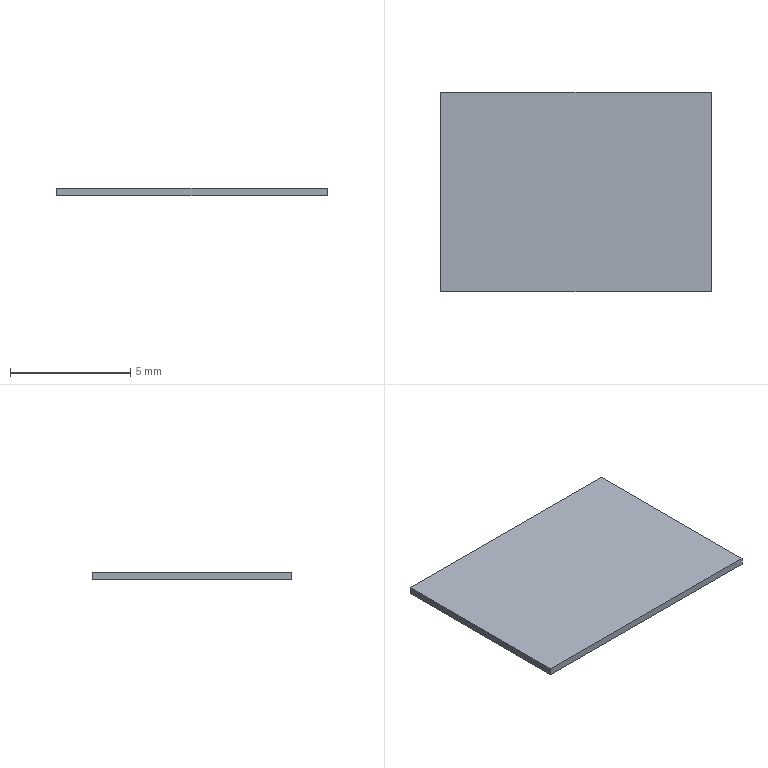Part | SolidWorks | features Extrusion 1 | 1 solid | 6 faces | box 11.25 x 8.29 x 0.3 mm | volume 27.979 mm3 | plane 6
STEP:
#1=CARTESIAN_POINT('',(5.625,-4.145,-0.15));
#2=VERTEX_POINT('',#1);
#3=CARTESIAN_POINT('',(5.625,4.145,-0.15));
#4=VERTEX_POINT('',#3);
#5=CARTESIAN_POINT('',(5.625,-4.145,-0.15));
#6=DIRECTION('',(0.,1.,0.));
#7=VECTOR('',#6,1000.);
#8=LINE('',#5,#7);
#9=EDGE_CURVE('',#2,#4,#8,.T.);
#10=ORIENTED_EDGE('',*,*,#9,.T.);
#11=CARTESIAN_POINT('',(5.625,4.145,0.15));
#12=VERTEX_POINT('',#11);
#13=CARTESIAN_POINT('',(5.625,4.145,0.15));
#14=DIRECTION('',(0.,0.,-1.));
#15=VECTOR('',#14,1000.);
#16=LINE('',#13,#15);
#17=EDGE_CURVE('',#12,#4,#16,.T.);
#18=ORIENTED_EDGE('',*,*,#17,.F.);
#19=CARTESIAN_POINT('',(5.625,-4.145,0.15));
#20=VERTEX_POINT('',#19);
#21=CARTESIAN_POINT('',(5.625,-4.145,0.15));
#22=DIRECTION('',(0.,1.,0.));
#23=VECTOR('',#22,1000.);
#24=LINE('',#21,#23);
#25=EDGE_CURVE('',#20,#12,#24,.T.);
#26=ORIENTED_EDGE('',*,*,#25,.F.);
#27=CARTESIAN_POINT('',(5.625,-4.145,0.15));
#28=DIRECTION('',(0.,0.,-1.));
#29=VECTOR('',#28,1000.);
#30=LINE('',#27,#29);
#31=EDGE_CURVE('',#20,#2,#30,.T.);
#32=ORIENTED_EDGE('',*,*,#31,.T.);
#33=EDGE_LOOP('',(#10,#18,#26,#32));
#34=FACE_OUTER_BOUND('',#33,.T.);
#35=CARTESIAN_POINT('',(5.625,-4.145,0.15));
#36=DIRECTION('',(-1.,0.,0.));
#37=DIRECTION('',(0.,0.,1.));
#38=AXIS2_PLACEMENT_3D('',#35,#36,#37);
#39=PLANE('',#38);
#40=ADVANCED_FACE('',(#34),#39,.F.);
#41=CARTESIAN_POINT('',(-5.625,4.145,-0.15));
#42=VERTEX_POINT('',#41);
#43=CARTESIAN_POINT('',(-5.625,4.145,-0.15));
#44=DIRECTION('',(-1.,0.,0.));
#45=VECTOR('',#44,1000.);
#46=LINE('',#43,#45);
#47=EDGE_CURVE('',#4,#42,#46,.T.);
#48=ORIENTED_EDGE('',*,*,#47,.T.);
#49=CARTESIAN_POINT('',(-5.625,4.145,0.15));
#50=VERTEX_POINT('',#49);
#51=CARTESIAN_POINT('',(-5.625,4.145,0.15));
#52=DIRECTION('',(0.,0.,-1.));
#53=VECTOR('',#52,1000.);
#54=LINE('',#51,#53);
#55=EDGE_CURVE('',#50,#42,#54,.T.);
#56=ORIENTED_EDGE('',*,*,#55,.F.);
#57=CARTESIAN_POINT('',(-5.625,4.145,0.15));
#58=DIRECTION('',(-1.,0.,0.));
#59=VECTOR('',#58,1000.);
#60=LINE('',#57,#59);
#61=EDGE_CURVE('',#12,#50,#60,.T.);
#62=ORIENTED_EDGE('',*,*,#61,.F.);
#63=ORIENTED_EDGE('',*,*,#17,.T.);
#64=EDGE_LOOP('',(#48,#56,#62,#63));
#65=FACE_OUTER_BOUND('',#64,.T.);
#66=CARTESIAN_POINT('',(-5.625,4.145,0.15));
#67=DIRECTION('',(0.,-1.,0.));
#68=DIRECTION('',(0.,0.,-1.));
#69=AXIS2_PLACEMENT_3D('',#66,#67,#68);
#70=PLANE('',#69);
#71=ADVANCED_FACE('',(#65),#70,.F.);
#72=CARTESIAN_POINT('',(-5.625,-4.145,-0.15));
#73=VERTEX_POINT('',#72);
#74=CARTESIAN_POINT('',(-5.625,-4.145,-0.15));
#75=DIRECTION('',(0.,-1.,0.));
#76=VECTOR('',#75,1000.);
#77=LINE('',#74,#76);
#78=EDGE_CURVE('',#42,#73,#77,.T.);
#79=ORIENTED_EDGE('',*,*,#78,.T.);
#80=CARTESIAN_POINT('',(-5.625,-4.145,0.15));
#81=VERTEX_POINT('',#80);
#82=CARTESIAN_POINT('',(-5.625,-4.145,0.15));
#83=DIRECTION('',(0.,0.,-1.));
#84=VECTOR('',#83,1000.);
#85=LINE('',#82,#84);
#86=EDGE_CURVE('',#81,#73,#85,.T.);
#87=ORIENTED_EDGE('',*,*,#86,.F.);
#88=CARTESIAN_POINT('',(-5.625,-4.145,0.15));
#89=DIRECTION('',(0.,-1.,0.));
#90=VECTOR('',#89,1000.);
#91=LINE('',#88,#90);
#92=EDGE_CURVE('',#50,#81,#91,.T.);
#93=ORIENTED_EDGE('',*,*,#92,.F.);
#94=ORIENTED_EDGE('',*,*,#55,.T.);
#95=EDGE_LOOP('',(#79,#87,#93,#94));
#96=FACE_OUTER_BOUND('',#95,.T.);
#97=CARTESIAN_POINT('',(-5.625,-4.145,0.15));
#98=DIRECTION('',(1.,0.,0.));
#99=DIRECTION('',(0.,0.,-1.));
#100=AXIS2_PLACEMENT_3D('',#97,#98,#99);
#101=PLANE('',#100);
#102=ADVANCED_FACE('',(#96),#101,.F.);
#103=CARTESIAN_POINT('',(-5.625,-4.145,-0.15));
#104=DIRECTION('',(1.,0.,0.));
#105=VECTOR('',#104,1000.);
#106=LINE('',#103,#105);
#107=EDGE_CURVE('',#73,#2,#106,.T.);
#108=ORIENTED_EDGE('',*,*,#107,.T.);
#109=ORIENTED_EDGE('',*,*,#31,.F.);
#110=CARTESIAN_POINT('',(-5.625,-4.145,0.15));
#111=DIRECTION('',(1.,0.,0.));
#112=VECTOR('',#111,1000.);
#113=LINE('',#110,#112);
#114=EDGE_CURVE('',#81,#20,#113,.T.);
#115=ORIENTED_EDGE('',*,*,#114,.F.);
#116=ORIENTED_EDGE('',*,*,#86,.T.);
#117=EDGE_LOOP('',(#108,#109,#115,#116));
#118=FACE_OUTER_BOUND('',#117,.T.);
#119=CARTESIAN_POINT('',(-5.625,-4.145,0.15));
#120=DIRECTION('',(0.,1.,0.));
#121=DIRECTION('',(0.,0.,1.));
#122=AXIS2_PLACEMENT_3D('',#119,#120,#121);
#123=PLANE('',#122);
#124=ADVANCED_FACE('',(#118),#123,.F.);
#125=ORIENTED_EDGE('',*,*,#25,.T.);
#126=ORIENTED_EDGE('',*,*,#61,.T.);
#127=ORIENTED_EDGE('',*,*,#92,.T.);
#128=ORIENTED_EDGE('',*,*,#114,.T.);
#129=EDGE_LOOP('',(#125,#126,#127,#128));
#130=FACE_OUTER_BOUND('',#129,.T.);
#131=CARTESIAN_POINT('',(0.,0.,0.15));
#132=DIRECTION('',(0.,0.,-1.));
#133=DIRECTION('',(-1.,0.,0.));
#134=AXIS2_PLACEMENT_3D('',#131,#132,#133);
#135=PLANE('',#134);
#136=ADVANCED_FACE('',(#130),#135,.F.);
#137=ORIENTED_EDGE('',*,*,#9,.F.);
#138=ORIENTED_EDGE('',*,*,#107,.F.);
#139=ORIENTED_EDGE('',*,*,#78,.F.);
#140=ORIENTED_EDGE('',*,*,#47,.F.);
#141=EDGE_LOOP('',(#137,#138,#139,#140));
#142=FACE_OUTER_BOUND('',#141,.T.);
#143=CARTESIAN_POINT('',(0.,0.,-0.15));
#144=DIRECTION('',(0.,0.,-1.));
#145=DIRECTION('',(-1.,0.,0.));
#146=AXIS2_PLACEMENT_3D('',#143,#144,#145);
#147=PLANE('',#146);
#148=ADVANCED_FACE('',(#142),#147,.T.);
#149=CLOSED_SHELL('',(#40,#71,#102,#124,#136,#148));
#150=MANIFOLD_SOLID_BREP('',#149);
#151=CARTESIAN_POINT('',(0.,0.,0.));
#152=DIRECTION('',(0.,0.,1.));
#153=DIRECTION('',(1.,0.,0.));
#154=AXIS2_PLACEMENT_3D('',#151,#152,#153);
#155=(LENGTH_UNIT()NAMED_UNIT(*)SI_UNIT(.MILLI.,.METRE.));
#156=UNCERTAINTY_MEASURE_WITH_UNIT(LENGTH_MEASURE(0.00001),#155,'','');
#157=(NAMED_UNIT(*)PLANE_ANGLE_UNIT()SI_UNIT($,.RADIAN.));
#158=(NAMED_UNIT(*)SI_UNIT($,.STERADIAN.)SOLID_ANGLE_UNIT());
#159=(GEOMETRIC_REPRESENTATION_CONTEXT(3)GLOBAL_UNCERTAINTY_ASSIGNED_CONTEXT((#156))GLOBAL_UNIT_ASSIGNED_CONTEXT((#155,#157,#158))REPRESENTATION_CONTEXT('',''));
#160=ADVANCED_BREP_SHAPE_REPRESENTATION('',(#150,#154),#159);